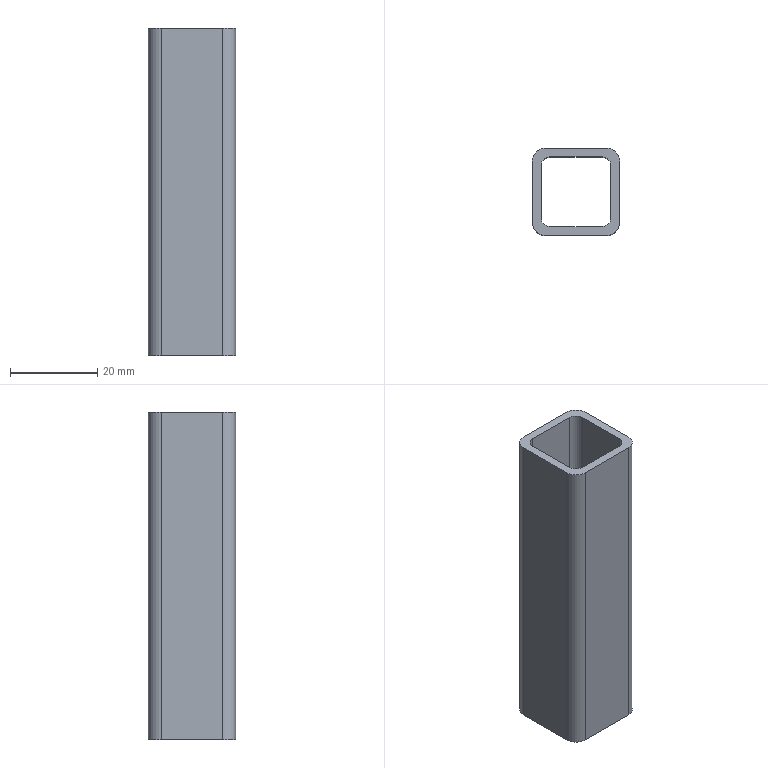Part | STEP file | DIN EN 10210-2 - 20 x 20 x 2 - 100 | 1 solid | 18 faces | box 20 x 20 x 75 mm | volume 10478 mm3 | plane 10 | cylinder 8 | commonest cylinder face diameters 4 x4 6 x4
STEP:
#1=CARTESIAN_POINT('',(0.,0.,0.));
#2=DIRECTION('',(0.,0.,1.));
#3=DIRECTION('',(1.,0.,0.));
#4=AXIS2_PLACEMENT_3D('',#1,#2,#3);
#5=CARTESIAN_POINT('',(8.,6.,0.));
#6=VERTEX_POINT('',#5);
#7=CARTESIAN_POINT('',(8.,6.,75.));
#8=VERTEX_POINT('',#7);
#9=CARTESIAN_POINT('',(8.,6.,0.));
#10=DIRECTION('',(0.,0.,1.));
#11=VECTOR('',#10,1.);
#12=LINE('',#9,#11);
#13=CARTESIAN_POINT('',(6.,6.,0.));
#14=DIRECTION('',(0.,0.,1.));
#15=DIRECTION('',(1.,0.,0.));
#16=AXIS2_PLACEMENT_3D('',#13,#14,#15);
#17=CYLINDRICAL_SURFACE('',#16,2.);
#18=CARTESIAN_POINT('',(0.,0.));
#19=DIRECTION('',(0.,1.));
#20=VECTOR('',#19,1.);
#21=LINE('',#18,#20);
#22=(GEOMETRIC_REPRESENTATION_CONTEXT(2)PARAMETRIC_REPRESENTATION_CONTEXT()REPRESENTATION_CONTEXT('',''));
#23=DEFINITIONAL_REPRESENTATION('',(#21),#22);
#24=PCURVE('',#17,#23);
#25=CARTESIAN_POINT('',(8.,6.,0.));
#26=DIRECTION('',(1.,0.,0.));
#27=DIRECTION('',(0.,0.,-1.));
#28=AXIS2_PLACEMENT_3D('',#25,#26,#27);
#29=PLANE('',#28);
#30=CARTESIAN_POINT('',(0.,0.));
#31=DIRECTION('',(-1.,0.));
#32=VECTOR('',#31,1.);
#33=LINE('',#30,#32);
#34=(GEOMETRIC_REPRESENTATION_CONTEXT(2)PARAMETRIC_REPRESENTATION_CONTEXT()REPRESENTATION_CONTEXT('',''));
#35=DEFINITIONAL_REPRESENTATION('',(#33),#34);
#36=PCURVE('',#29,#35);
#37=SURFACE_CURVE('',#12,(#24,#36),.PCURVE_S1.);
#38=EDGE_CURVE('',#6,#8,#37,.T.);
#39=ORIENTED_EDGE('',*,*,#38,.F.);
#40=CARTESIAN_POINT('',(6.,8.,0.));
#41=VERTEX_POINT('',#40);
#42=CARTESIAN_POINT('',(6.,6.,0.));
#43=DIRECTION('',(0.,0.,1.));
#44=DIRECTION('',(1.,0.,0.));
#45=AXIS2_PLACEMENT_3D('',#42,#43,#44);
#46=CIRCLE('',#45,2.);
#47=CARTESIAN_POINT('',(0.,0.));
#48=DIRECTION('',(1.,0.));
#49=VECTOR('',#48,1.);
#50=LINE('',#47,#49);
#51=(GEOMETRIC_REPRESENTATION_CONTEXT(2)PARAMETRIC_REPRESENTATION_CONTEXT()REPRESENTATION_CONTEXT('',''));
#52=DEFINITIONAL_REPRESENTATION('',(#50),#51);
#53=PCURVE('',#17,#52);
#54=CARTESIAN_POINT('',(0.,0.,0.));
#55=DIRECTION('',(0.,0.,1.));
#56=DIRECTION('',(1.,0.,0.));
#57=AXIS2_PLACEMENT_3D('',#54,#55,#56);
#58=PLANE('',#57);
#59=CARTESIAN_POINT('',(6.,6.));
#60=DIRECTION('',(1.,0.));
#61=AXIS2_PLACEMENT_2D('',#59,#60);
#62=CIRCLE('',#61,2.);
#63=(GEOMETRIC_REPRESENTATION_CONTEXT(2)PARAMETRIC_REPRESENTATION_CONTEXT()REPRESENTATION_CONTEXT('',''));
#64=DEFINITIONAL_REPRESENTATION('',(#62),#63);
#65=PCURVE('',#58,#64);
#66=SURFACE_CURVE('',#46,(#53,#65),.PCURVE_S1.);
#67=EDGE_CURVE('',#6,#41,#66,.T.);
#68=ORIENTED_EDGE('',*,*,#67,.T.);
#69=CARTESIAN_POINT('',(6.,8.,75.));
#70=VERTEX_POINT('',#69);
#71=CARTESIAN_POINT('',(6.,8.,0.));
#72=DIRECTION('',(0.,0.,1.));
#73=VECTOR('',#72,1.);
#74=LINE('',#71,#73);
#75=CARTESIAN_POINT('',(1.571,0.));
#76=DIRECTION('',(0.,1.));
#77=VECTOR('',#76,1.);
#78=LINE('',#75,#77);
#79=(GEOMETRIC_REPRESENTATION_CONTEXT(2)PARAMETRIC_REPRESENTATION_CONTEXT()REPRESENTATION_CONTEXT('',''));
#80=DEFINITIONAL_REPRESENTATION('',(#78),#79);
#81=PCURVE('',#17,#80);
#82=CARTESIAN_POINT('',(-6.,8.,0.));
#83=DIRECTION('',(0.,1.,0.));
#84=DIRECTION('',(0.,0.,1.));
#85=AXIS2_PLACEMENT_3D('',#82,#83,#84);
#86=PLANE('',#85);
#87=CARTESIAN_POINT('',(0.,12.));
#88=DIRECTION('',(1.,0.));
#89=VECTOR('',#88,1.);
#90=LINE('',#87,#89);
#91=(GEOMETRIC_REPRESENTATION_CONTEXT(2)PARAMETRIC_REPRESENTATION_CONTEXT()REPRESENTATION_CONTEXT('',''));
#92=DEFINITIONAL_REPRESENTATION('',(#90),#91);
#93=PCURVE('',#86,#92);
#94=SURFACE_CURVE('',#74,(#81,#93),.PCURVE_S1.);
#95=EDGE_CURVE('',#41,#70,#94,.T.);
#96=ORIENTED_EDGE('',*,*,#95,.T.);
#97=CARTESIAN_POINT('',(6.,6.,75.));
#98=DIRECTION('',(0.,0.,1.));
#99=DIRECTION('',(1.,0.,0.));
#100=AXIS2_PLACEMENT_3D('',#97,#98,#99);
#101=CIRCLE('',#100,2.);
#102=CARTESIAN_POINT('',(0.,75.));
#103=DIRECTION('',(1.,0.));
#104=VECTOR('',#103,1.);
#105=LINE('',#102,#104);
#106=(GEOMETRIC_REPRESENTATION_CONTEXT(2)PARAMETRIC_REPRESENTATION_CONTEXT()REPRESENTATION_CONTEXT('',''));
#107=DEFINITIONAL_REPRESENTATION('',(#105),#106);
#108=PCURVE('',#17,#107);
#109=CARTESIAN_POINT('',(0.,0.,75.));
#110=DIRECTION('',(0.,0.,1.));
#111=DIRECTION('',(1.,0.,0.));
#112=AXIS2_PLACEMENT_3D('',#109,#110,#111);
#113=PLANE('',#112);
#114=CARTESIAN_POINT('',(6.,6.));
#115=DIRECTION('',(1.,0.));
#116=AXIS2_PLACEMENT_2D('',#114,#115);
#117=CIRCLE('',#116,2.);
#118=(GEOMETRIC_REPRESENTATION_CONTEXT(2)PARAMETRIC_REPRESENTATION_CONTEXT()REPRESENTATION_CONTEXT('',''));
#119=DEFINITIONAL_REPRESENTATION('',(#117),#118);
#120=PCURVE('',#113,#119);
#121=SURFACE_CURVE('',#101,(#108,#120),.PCURVE_S1.);
#122=EDGE_CURVE('',#8,#70,#121,.T.);
#123=ORIENTED_EDGE('',*,*,#122,.F.);
#124=EDGE_LOOP('',(#39,#68,#96,#123));
#125=FACE_BOUND('',#124,.F.);
#126=ADVANCED_FACE('',(#125),#17,.F.);
#127=CARTESIAN_POINT('',(-6.,8.,75.));
#128=VERTEX_POINT('',#127);
#129=CARTESIAN_POINT('',(-3.,8.,75.));
#130=DIRECTION('',(-1.,0.,0.));
#131=VECTOR('',#130,1.);
#132=LINE('',#129,#131);
#133=CARTESIAN_POINT('',(75.,3.));
#134=DIRECTION('',(0.,-1.));
#135=VECTOR('',#134,1.);
#136=LINE('',#133,#135);
#137=(GEOMETRIC_REPRESENTATION_CONTEXT(2)PARAMETRIC_REPRESENTATION_CONTEXT()REPRESENTATION_CONTEXT('',''));
#138=DEFINITIONAL_REPRESENTATION('',(#136),#137);
#139=PCURVE('',#86,#138);
#140=CARTESIAN_POINT('',(-3.,8.));
#141=DIRECTION('',(-1.,0.));
#142=VECTOR('',#141,1.);
#143=LINE('',#140,#142);
#144=(GEOMETRIC_REPRESENTATION_CONTEXT(2)PARAMETRIC_REPRESENTATION_CONTEXT()REPRESENTATION_CONTEXT('',''));
#145=DEFINITIONAL_REPRESENTATION('',(#143),#144);
#146=PCURVE('',#113,#145);
#147=SURFACE_CURVE('',#132,(#139,#146),.PCURVE_S1.);
#148=EDGE_CURVE('',#70,#128,#147,.T.);
#149=ORIENTED_EDGE('',*,*,#148,.T.);
#150=CARTESIAN_POINT('',(-6.,8.,0.));
#151=VERTEX_POINT('',#150);
#152=CARTESIAN_POINT('',(-6.,8.,0.));
#153=DIRECTION('',(0.,0.,1.));
#154=VECTOR('',#153,1.);
#155=LINE('',#152,#154);
#156=CARTESIAN_POINT('',(0.,0.));
#157=DIRECTION('',(1.,0.));
#158=VECTOR('',#157,1.);
#159=LINE('',#156,#158);
#160=(GEOMETRIC_REPRESENTATION_CONTEXT(2)PARAMETRIC_REPRESENTATION_CONTEXT()REPRESENTATION_CONTEXT('',''));
#161=DEFINITIONAL_REPRESENTATION('',(#159),#160);
#162=PCURVE('',#86,#161);
#163=CARTESIAN_POINT('',(-6.,6.,0.));
#164=DIRECTION('',(0.,0.,1.));
#165=DIRECTION('',(0.,1.,0.));
#166=AXIS2_PLACEMENT_3D('',#163,#164,#165);
#167=CYLINDRICAL_SURFACE('',#166,2.);
#168=CARTESIAN_POINT('',(0.,0.));
#169=DIRECTION('',(0.,1.));
#170=VECTOR('',#169,1.);
#171=LINE('',#168,#170);
#172=(GEOMETRIC_REPRESENTATION_CONTEXT(2)PARAMETRIC_REPRESENTATION_CONTEXT()REPRESENTATION_CONTEXT('',''));
#173=DEFINITIONAL_REPRESENTATION('',(#171),#172);
#174=PCURVE('',#167,#173);
#175=SURFACE_CURVE('',#155,(#162,#174),.PCURVE_S1.);
#176=EDGE_CURVE('',#151,#128,#175,.T.);
#177=ORIENTED_EDGE('',*,*,#176,.F.);
#178=CARTESIAN_POINT('',(-3.,8.,0.));
#179=DIRECTION('',(-1.,0.,0.));
#180=VECTOR('',#179,1.);
#181=LINE('',#178,#180);
#182=CARTESIAN_POINT('',(0.,3.));
#183=DIRECTION('',(0.,-1.));
#184=VECTOR('',#183,1.);
#185=LINE('',#182,#184);
#186=(GEOMETRIC_REPRESENTATION_CONTEXT(2)PARAMETRIC_REPRESENTATION_CONTEXT()REPRESENTATION_CONTEXT('',''));
#187=DEFINITIONAL_REPRESENTATION('',(#185),#186);
#188=PCURVE('',#86,#187);
#189=CARTESIAN_POINT('',(-3.,8.));
#190=DIRECTION('',(-1.,0.));
#191=VECTOR('',#190,1.);
#192=LINE('',#189,#191);
#193=(GEOMETRIC_REPRESENTATION_CONTEXT(2)PARAMETRIC_REPRESENTATION_CONTEXT()REPRESENTATION_CONTEXT('',''));
#194=DEFINITIONAL_REPRESENTATION('',(#192),#193);
#195=PCURVE('',#58,#194);
#196=SURFACE_CURVE('',#181,(#188,#195),.PCURVE_S1.);
#197=EDGE_CURVE('',#41,#151,#196,.T.);
#198=ORIENTED_EDGE('',*,*,#197,.F.);
#199=ORIENTED_EDGE('',*,*,#95,.T.);
#200=EDGE_LOOP('',(#149,#177,#198,#199));
#201=FACE_BOUND('',#200,.T.);
#202=ADVANCED_FACE('',(#201),#86,.F.);
#203=ORIENTED_EDGE('',*,*,#176,.F.);
#204=CARTESIAN_POINT('',(-8.,6.,0.));
#205=VERTEX_POINT('',#204);
#206=CARTESIAN_POINT('',(-6.,6.,0.));
#207=DIRECTION('',(0.,0.,1.));
#208=DIRECTION('',(0.,1.,0.));
#209=AXIS2_PLACEMENT_3D('',#206,#207,#208);
#210=CIRCLE('',#209,2.);
#211=CARTESIAN_POINT('',(0.,0.));
#212=DIRECTION('',(1.,0.));
#213=VECTOR('',#212,1.);
#214=LINE('',#211,#213);
#215=(GEOMETRIC_REPRESENTATION_CONTEXT(2)PARAMETRIC_REPRESENTATION_CONTEXT()REPRESENTATION_CONTEXT('',''));
#216=DEFINITIONAL_REPRESENTATION('',(#214),#215);
#217=PCURVE('',#167,#216);
#218=CARTESIAN_POINT('',(-6.,6.));
#219=DIRECTION('',(0.,1.));
#220=AXIS2_PLACEMENT_2D('',#218,#219);
#221=CIRCLE('',#220,2.);
#222=(GEOMETRIC_REPRESENTATION_CONTEXT(2)PARAMETRIC_REPRESENTATION_CONTEXT()REPRESENTATION_CONTEXT('',''));
#223=DEFINITIONAL_REPRESENTATION('',(#221),#222);
#224=PCURVE('',#58,#223);
#225=SURFACE_CURVE('',#210,(#217,#224),.PCURVE_S1.);
#226=EDGE_CURVE('',#151,#205,#225,.T.);
#227=ORIENTED_EDGE('',*,*,#226,.T.);
#228=CARTESIAN_POINT('',(-8.,6.,75.));
#229=VERTEX_POINT('',#228);
#230=CARTESIAN_POINT('',(-8.,6.,0.));
#231=DIRECTION('',(0.,0.,1.));
#232=VECTOR('',#231,1.);
#233=LINE('',#230,#232);
#234=CARTESIAN_POINT('',(1.571,0.));
#235=DIRECTION('',(0.,1.));
#236=VECTOR('',#235,1.);
#237=LINE('',#234,#236);
#238=(GEOMETRIC_REPRESENTATION_CONTEXT(2)PARAMETRIC_REPRESENTATION_CONTEXT()REPRESENTATION_CONTEXT('',''));
#239=DEFINITIONAL_REPRESENTATION('',(#237),#238);
#240=PCURVE('',#167,#239);
#241=CARTESIAN_POINT('',(-8.,-6.,0.));
#242=DIRECTION('',(-1.,0.,0.));
#243=DIRECTION('',(0.,0.,1.));
#244=AXIS2_PLACEMENT_3D('',#241,#242,#243);
#245=PLANE('',#244);
#246=CARTESIAN_POINT('',(0.,12.));
#247=DIRECTION('',(1.,0.));
#248=VECTOR('',#247,1.);
#249=LINE('',#246,#248);
#250=(GEOMETRIC_REPRESENTATION_CONTEXT(2)PARAMETRIC_REPRESENTATION_CONTEXT()REPRESENTATION_CONTEXT('',''));
#251=DEFINITIONAL_REPRESENTATION('',(#249),#250);
#252=PCURVE('',#245,#251);
#253=SURFACE_CURVE('',#233,(#240,#252),.PCURVE_S1.);
#254=EDGE_CURVE('',#205,#229,#253,.T.);
#255=ORIENTED_EDGE('',*,*,#254,.T.);
#256=CARTESIAN_POINT('',(-6.,6.,75.));
#257=DIRECTION('',(0.,0.,1.));
#258=DIRECTION('',(0.,1.,0.));
#259=AXIS2_PLACEMENT_3D('',#256,#257,#258);
#260=CIRCLE('',#259,2.);
#261=CARTESIAN_POINT('',(0.,75.));
#262=DIRECTION('',(1.,0.));
#263=VECTOR('',#262,1.);
#264=LINE('',#261,#263);
#265=(GEOMETRIC_REPRESENTATION_CONTEXT(2)PARAMETRIC_REPRESENTATION_CONTEXT()REPRESENTATION_CONTEXT('',''));
#266=DEFINITIONAL_REPRESENTATION('',(#264),#265);
#267=PCURVE('',#167,#266);
#268=CARTESIAN_POINT('',(-6.,6.));
#269=DIRECTION('',(0.,1.));
#270=AXIS2_PLACEMENT_2D('',#268,#269);
#271=CIRCLE('',#270,2.);
#272=(GEOMETRIC_REPRESENTATION_CONTEXT(2)PARAMETRIC_REPRESENTATION_CONTEXT()REPRESENTATION_CONTEXT('',''));
#273=DEFINITIONAL_REPRESENTATION('',(#271),#272);
#274=PCURVE('',#113,#273);
#275=SURFACE_CURVE('',#260,(#267,#274),.PCURVE_S1.);
#276=EDGE_CURVE('',#128,#229,#275,.T.);
#277=ORIENTED_EDGE('',*,*,#276,.F.);
#278=EDGE_LOOP('',(#203,#227,#255,#277));
#279=FACE_BOUND('',#278,.F.);
#280=ADVANCED_FACE('',(#279),#167,.F.);
#281=CARTESIAN_POINT('',(-8.,-6.,75.));
#282=VERTEX_POINT('',#281);
#283=CARTESIAN_POINT('',(-8.,-3.,75.));
#284=DIRECTION('',(0.,-1.,0.));
#285=VECTOR('',#284,1.);
#286=LINE('',#283,#285);
#287=CARTESIAN_POINT('',(75.,3.));
#288=DIRECTION('',(0.,-1.));
#289=VECTOR('',#288,1.);
#290=LINE('',#287,#289);
#291=(GEOMETRIC_REPRESENTATION_CONTEXT(2)PARAMETRIC_REPRESENTATION_CONTEXT()REPRESENTATION_CONTEXT('',''));
#292=DEFINITIONAL_REPRESENTATION('',(#290),#291);
#293=PCURVE('',#245,#292);
#294=CARTESIAN_POINT('',(-8.,-3.));
#295=DIRECTION('',(0.,-1.));
#296=VECTOR('',#295,1.);
#297=LINE('',#294,#296);
#298=(GEOMETRIC_REPRESENTATION_CONTEXT(2)PARAMETRIC_REPRESENTATION_CONTEXT()REPRESENTATION_CONTEXT('',''));
#299=DEFINITIONAL_REPRESENTATION('',(#297),#298);
#300=PCURVE('',#113,#299);
#301=SURFACE_CURVE('',#286,(#293,#300),.PCURVE_S1.);
#302=EDGE_CURVE('',#229,#282,#301,.T.);
#303=ORIENTED_EDGE('',*,*,#302,.T.);
#304=CARTESIAN_POINT('',(-8.,-6.,0.));
#305=VERTEX_POINT('',#304);
#306=CARTESIAN_POINT('',(-8.,-6.,0.));
#307=DIRECTION('',(0.,0.,1.));
#308=VECTOR('',#307,1.);
#309=LINE('',#306,#308);
#310=CARTESIAN_POINT('',(0.,0.));
#311=DIRECTION('',(1.,0.));
#312=VECTOR('',#311,1.);
#313=LINE('',#310,#312);
#314=(GEOMETRIC_REPRESENTATION_CONTEXT(2)PARAMETRIC_REPRESENTATION_CONTEXT()REPRESENTATION_CONTEXT('',''));
#315=DEFINITIONAL_REPRESENTATION('',(#313),#314);
#316=PCURVE('',#245,#315);
#317=CARTESIAN_POINT('',(-6.,-6.,0.));
#318=DIRECTION('',(0.,0.,1.));
#319=DIRECTION('',(-1.,0.,0.));
#320=AXIS2_PLACEMENT_3D('',#317,#318,#319);
#321=CYLINDRICAL_SURFACE('',#320,2.);
#322=CARTESIAN_POINT('',(0.,0.));
#323=DIRECTION('',(0.,1.));
#324=VECTOR('',#323,1.);
#325=LINE('',#322,#324);
#326=(GEOMETRIC_REPRESENTATION_CONTEXT(2)PARAMETRIC_REPRESENTATION_CONTEXT()REPRESENTATION_CONTEXT('',''));
#327=DEFINITIONAL_REPRESENTATION('',(#325),#326);
#328=PCURVE('',#321,#327);
#329=SURFACE_CURVE('',#309,(#316,#328),.PCURVE_S1.);
#330=EDGE_CURVE('',#305,#282,#329,.T.);
#331=ORIENTED_EDGE('',*,*,#330,.F.);
#332=CARTESIAN_POINT('',(-8.,-3.,0.));
#333=DIRECTION('',(0.,-1.,0.));
#334=VECTOR('',#333,1.);
#335=LINE('',#332,#334);
#336=CARTESIAN_POINT('',(0.,3.));
#337=DIRECTION('',(0.,-1.));
#338=VECTOR('',#337,1.);
#339=LINE('',#336,#338);
#340=(GEOMETRIC_REPRESENTATION_CONTEXT(2)PARAMETRIC_REPRESENTATION_CONTEXT()REPRESENTATION_CONTEXT('',''));
#341=DEFINITIONAL_REPRESENTATION('',(#339),#340);
#342=PCURVE('',#245,#341);
#343=CARTESIAN_POINT('',(-8.,-3.));
#344=DIRECTION('',(0.,-1.));
#345=VECTOR('',#344,1.);
#346=LINE('',#343,#345);
#347=(GEOMETRIC_REPRESENTATION_CONTEXT(2)PARAMETRIC_REPRESENTATION_CONTEXT()REPRESENTATION_CONTEXT('',''));
#348=DEFINITIONAL_REPRESENTATION('',(#346),#347);
#349=PCURVE('',#58,#348);
#350=SURFACE_CURVE('',#335,(#342,#349),.PCURVE_S1.);
#351=EDGE_CURVE('',#205,#305,#350,.T.);
#352=ORIENTED_EDGE('',*,*,#351,.F.);
#353=ORIENTED_EDGE('',*,*,#254,.T.);
#354=EDGE_LOOP('',(#303,#331,#352,#353));
#355=FACE_BOUND('',#354,.T.);
#356=ADVANCED_FACE('',(#355),#245,.F.);
#357=CARTESIAN_POINT('',(10.,7.,75.));
#358=VERTEX_POINT('',#357);
#359=CARTESIAN_POINT('',(10.,-7.,75.));
#360=VERTEX_POINT('',#359);
#361=CARTESIAN_POINT('',(10.,3.5,75.));
#362=DIRECTION('',(0.,-1.,0.));
#363=VECTOR('',#362,1.);
#364=LINE('',#361,#363);
#365=CARTESIAN_POINT('',(10.,7.,0.));
#366=DIRECTION('',(1.,0.,0.));
#367=DIRECTION('',(0.,0.,-1.));
#368=AXIS2_PLACEMENT_3D('',#365,#366,#367);
#369=PLANE('',#368);
#370=CARTESIAN_POINT('',(-75.,-3.5));
#371=DIRECTION('',(0.,-1.));
#372=VECTOR('',#371,1.);
#373=LINE('',#370,#372);
#374=(GEOMETRIC_REPRESENTATION_CONTEXT(2)PARAMETRIC_REPRESENTATION_CONTEXT()REPRESENTATION_CONTEXT('',''));
#375=DEFINITIONAL_REPRESENTATION('',(#373),#374);
#376=PCURVE('',#369,#375);
#377=CARTESIAN_POINT('',(10.,3.5));
#378=DIRECTION('',(0.,-1.));
#379=VECTOR('',#378,1.);
#380=LINE('',#377,#379);
#381=(GEOMETRIC_REPRESENTATION_CONTEXT(2)PARAMETRIC_REPRESENTATION_CONTEXT()REPRESENTATION_CONTEXT('',''));
#382=DEFINITIONAL_REPRESENTATION('',(#380),#381);
#383=PCURVE('',#113,#382);
#384=SURFACE_CURVE('',#364,(#376,#383),.PCURVE_S1.);
#385=EDGE_CURVE('',#358,#360,#384,.T.);
#386=ORIENTED_EDGE('',*,*,#385,.T.);
#387=CARTESIAN_POINT('',(10.,-7.,0.));
#388=VERTEX_POINT('',#387);
#389=CARTESIAN_POINT('',(10.,-7.,0.));
#390=DIRECTION('',(0.,0.,1.));
#391=VECTOR('',#390,1.);
#392=LINE('',#389,#391);
#393=CARTESIAN_POINT('',(0.,-14.));
#394=DIRECTION('',(-1.,0.));
#395=VECTOR('',#394,1.);
#396=LINE('',#393,#395);
#397=(GEOMETRIC_REPRESENTATION_CONTEXT(2)PARAMETRIC_REPRESENTATION_CONTEXT()REPRESENTATION_CONTEXT('',''));
#398=DEFINITIONAL_REPRESENTATION('',(#396),#397);
#399=PCURVE('',#369,#398);
#400=CARTESIAN_POINT('',(7.,-7.,0.));
#401=DIRECTION('',(0.,0.,1.));
#402=DIRECTION('',(0.,1.,0.));
#403=AXIS2_PLACEMENT_3D('',#400,#401,#402);
#404=CYLINDRICAL_SURFACE('',#403,3.);
#405=CARTESIAN_POINT('',(4.712,0.));
#406=DIRECTION('',(0.,1.));
#407=VECTOR('',#406,1.);
#408=LINE('',#405,#407);
#409=(GEOMETRIC_REPRESENTATION_CONTEXT(2)PARAMETRIC_REPRESENTATION_CONTEXT()REPRESENTATION_CONTEXT('',''));
#410=DEFINITIONAL_REPRESENTATION('',(#408),#409);
#411=PCURVE('',#404,#410);
#412=SURFACE_CURVE('',#392,(#399,#411),.PCURVE_S1.);
#413=EDGE_CURVE('',#388,#360,#412,.T.);
#414=ORIENTED_EDGE('',*,*,#413,.F.);
#415=CARTESIAN_POINT('',(10.,7.,0.));
#416=VERTEX_POINT('',#415);
#417=CARTESIAN_POINT('',(10.,3.5,0.));
#418=DIRECTION('',(0.,-1.,0.));
#419=VECTOR('',#418,1.);
#420=LINE('',#417,#419);
#421=CARTESIAN_POINT('',(0.,-3.5));
#422=DIRECTION('',(0.,-1.));
#423=VECTOR('',#422,1.);
#424=LINE('',#421,#423);
#425=(GEOMETRIC_REPRESENTATION_CONTEXT(2)PARAMETRIC_REPRESENTATION_CONTEXT()REPRESENTATION_CONTEXT('',''));
#426=DEFINITIONAL_REPRESENTATION('',(#424),#425);
#427=PCURVE('',#369,#426);
#428=CARTESIAN_POINT('',(10.,3.5));
#429=DIRECTION('',(0.,-1.));
#430=VECTOR('',#429,1.);
#431=LINE('',#428,#430);
#432=(GEOMETRIC_REPRESENTATION_CONTEXT(2)PARAMETRIC_REPRESENTATION_CONTEXT()REPRESENTATION_CONTEXT('',''));
#433=DEFINITIONAL_REPRESENTATION('',(#431),#432);
#434=PCURVE('',#58,#433);
#435=SURFACE_CURVE('',#420,(#427,#434),.PCURVE_S1.);
#436=EDGE_CURVE('',#416,#388,#435,.T.);
#437=ORIENTED_EDGE('',*,*,#436,.F.);
#438=CARTESIAN_POINT('',(10.,7.,0.));
#439=DIRECTION('',(0.,0.,1.));
#440=VECTOR('',#439,1.);
#441=LINE('',#438,#440);
#442=CARTESIAN_POINT('',(0.,0.));
#443=DIRECTION('',(-1.,0.));
#444=VECTOR('',#443,1.);
#445=LINE('',#442,#444);
#446=(GEOMETRIC_REPRESENTATION_CONTEXT(2)PARAMETRIC_REPRESENTATION_CONTEXT()REPRESENTATION_CONTEXT('',''));
#447=DEFINITIONAL_REPRESENTATION('',(#445),#446);
#448=PCURVE('',#369,#447);
#449=CARTESIAN_POINT('',(7.,7.,0.));
#450=DIRECTION('',(0.,0.,1.));
#451=DIRECTION('',(-1.,0.,0.));
#452=AXIS2_PLACEMENT_3D('',#449,#450,#451);
#453=CYLINDRICAL_SURFACE('',#452,3.);
#454=CARTESIAN_POINT('',(3.142,0.));
#455=DIRECTION('',(0.,1.));
#456=VECTOR('',#455,1.);
#457=LINE('',#454,#456);
#458=(GEOMETRIC_REPRESENTATION_CONTEXT(2)PARAMETRIC_REPRESENTATION_CONTEXT()REPRESENTATION_CONTEXT('',''));
#459=DEFINITIONAL_REPRESENTATION('',(#457),#458);
#460=PCURVE('',#453,#459);
#461=SURFACE_CURVE('',#441,(#448,#460),.PCURVE_S1.);
#462=EDGE_CURVE('',#416,#358,#461,.T.);
#463=ORIENTED_EDGE('',*,*,#462,.T.);
#464=EDGE_LOOP('',(#386,#414,#437,#463));
#465=FACE_BOUND('',#464,.T.);
#466=ADVANCED_FACE('',(#465),#369,.T.);
#467=CARTESIAN_POINT('',(7.,-10.,75.));
#468=VERTEX_POINT('',#467);
#469=CARTESIAN_POINT('',(7.,-7.,75.));
#470=DIRECTION('',(0.,0.,-1.));
#471=DIRECTION('',(0.,1.,0.));
#472=AXIS2_PLACEMENT_3D('',#469,#470,#471);
#473=CIRCLE('',#472,3.);
#474=CARTESIAN_POINT('',(6.283,75.));
#475=DIRECTION('',(-1.,0.));
#476=VECTOR('',#475,1.);
#477=LINE('',#474,#476);
#478=(GEOMETRIC_REPRESENTATION_CONTEXT(2)PARAMETRIC_REPRESENTATION_CONTEXT()REPRESENTATION_CONTEXT('',''));
#479=DEFINITIONAL_REPRESENTATION('',(#477),#478);
#480=PCURVE('',#404,#479);
#481=CARTESIAN_POINT('',(7.,-4.));
#482=CARTESIAN_POINT('',(12.196,-4.));
#483=CARTESIAN_POINT('',(9.598,-8.5));
#484=CARTESIAN_POINT('',(7.,-13.));
#485=CARTESIAN_POINT('',(4.402,-8.5));
#486=CARTESIAN_POINT('',(1.804,-4.));
#487=CARTESIAN_POINT('',(7.,-4.));
#488=(BOUNDED_CURVE()B_SPLINE_CURVE(2,(#481,#482,#483,#484,#485,#486,#487),.UNSPECIFIED.,.T.,.F.)B_SPLINE_CURVE_WITH_KNOTS((1,2,2,2,2,1),(-2.094,0.,2.094,4.189,6.283,8.378),.UNSPECIFIED.)CURVE()GEOMETRIC_REPRESENTATION_ITEM()RATIONAL_B_SPLINE_CURVE((1.,0.5,1.,0.5,1.,0.5,1.))REPRESENTATION_ITEM(''));
#489=(GEOMETRIC_REPRESENTATION_CONTEXT(2)PARAMETRIC_REPRESENTATION_CONTEXT()REPRESENTATION_CONTEXT('',''));
#490=DEFINITIONAL_REPRESENTATION('',(#488),#489);
#491=PCURVE('',#113,#490);
#492=SURFACE_CURVE('',#473,(#480,#491),.PCURVE_S1.);
#493=EDGE_CURVE('',#360,#468,#492,.T.);
#494=ORIENTED_EDGE('',*,*,#493,.T.);
#495=CARTESIAN_POINT('',(7.,-10.,0.));
#496=VERTEX_POINT('',#495);
#497=CARTESIAN_POINT('',(7.,-10.,0.));
#498=DIRECTION('',(0.,0.,1.));
#499=VECTOR('',#498,1.);
#500=LINE('',#497,#499);
#501=CARTESIAN_POINT('',(3.142,0.));
#502=DIRECTION('',(0.,1.));
#503=VECTOR('',#502,1.);
#504=LINE('',#501,#503);
#505=(GEOMETRIC_REPRESENTATION_CONTEXT(2)PARAMETRIC_REPRESENTATION_CONTEXT()REPRESENTATION_CONTEXT('',''));
#506=DEFINITIONAL_REPRESENTATION('',(#504),#505);
#507=PCURVE('',#404,#506);
#508=CARTESIAN_POINT('',(7.,-10.,0.));
#509=DIRECTION('',(0.,-1.,0.));
#510=DIRECTION('',(0.,0.,-1.));
#511=AXIS2_PLACEMENT_3D('',#508,#509,#510);
#512=PLANE('',#511);
#513=CARTESIAN_POINT('',(0.,0.));
#514=DIRECTION('',(-1.,0.));
#515=VECTOR('',#514,1.);
#516=LINE('',#513,#515);
#517=(GEOMETRIC_REPRESENTATION_CONTEXT(2)PARAMETRIC_REPRESENTATION_CONTEXT()REPRESENTATION_CONTEXT('',''));
#518=DEFINITIONAL_REPRESENTATION('',(#516),#517);
#519=PCURVE('',#512,#518);
#520=SURFACE_CURVE('',#500,(#507,#519),.PCURVE_S1.);
#521=EDGE_CURVE('',#496,#468,#520,.T.);
#522=ORIENTED_EDGE('',*,*,#521,.F.);
#523=CARTESIAN_POINT('',(7.,-7.,0.));
#524=DIRECTION('',(0.,0.,-1.));
#525=DIRECTION('',(0.,1.,0.));
#526=AXIS2_PLACEMENT_3D('',#523,#524,#525);
#527=CIRCLE('',#526,3.);
#528=CARTESIAN_POINT('',(6.283,0.));
#529=DIRECTION('',(-1.,0.));
#530=VECTOR('',#529,1.);
#531=LINE('',#528,#530);
#532=(GEOMETRIC_REPRESENTATION_CONTEXT(2)PARAMETRIC_REPRESENTATION_CONTEXT()REPRESENTATION_CONTEXT('',''));
#533=DEFINITIONAL_REPRESENTATION('',(#531),#532);
#534=PCURVE('',#404,#533);
#535=CARTESIAN_POINT('',(7.,-4.));
#536=CARTESIAN_POINT('',(12.196,-4.));
#537=CARTESIAN_POINT('',(9.598,-8.5));
#538=CARTESIAN_POINT('',(7.,-13.));
#539=CARTESIAN_POINT('',(4.402,-8.5));
#540=CARTESIAN_POINT('',(1.804,-4.));
#541=CARTESIAN_POINT('',(7.,-4.));
#542=(BOUNDED_CURVE()B_SPLINE_CURVE(2,(#535,#536,#537,#538,#539,#540,#541),.UNSPECIFIED.,.T.,.F.)B_SPLINE_CURVE_WITH_KNOTS((1,2,2,2,2,1),(-2.094,0.,2.094,4.189,6.283,8.378),.UNSPECIFIED.)CURVE()GEOMETRIC_REPRESENTATION_ITEM()RATIONAL_B_SPLINE_CURVE((1.,0.5,1.,0.5,1.,0.5,1.))REPRESENTATION_ITEM(''));
#543=(GEOMETRIC_REPRESENTATION_CONTEXT(2)PARAMETRIC_REPRESENTATION_CONTEXT()REPRESENTATION_CONTEXT('',''));
#544=DEFINITIONAL_REPRESENTATION('',(#542),#543);
#545=PCURVE('',#58,#544);
#546=SURFACE_CURVE('',#527,(#534,#545),.PCURVE_S1.);
#547=EDGE_CURVE('',#388,#496,#546,.T.);
#548=ORIENTED_EDGE('',*,*,#547,.F.);
#549=ORIENTED_EDGE('',*,*,#413,.T.);
#550=EDGE_LOOP('',(#494,#522,#548,#549));
#551=FACE_BOUND('',#550,.T.);
#552=ADVANCED_FACE('',(#551),#404,.T.);
#553=CARTESIAN_POINT('',(-7.,-10.,75.));
#554=VERTEX_POINT('',#553);
#555=CARTESIAN_POINT('',(3.5,-10.,75.));
#556=DIRECTION('',(-1.,0.,0.));
#557=VECTOR('',#556,1.);
#558=LINE('',#555,#557);
#559=CARTESIAN_POINT('',(-75.,-3.5));
#560=DIRECTION('',(0.,-1.));
#561=VECTOR('',#560,1.);
#562=LINE('',#559,#561);
#563=(GEOMETRIC_REPRESENTATION_CONTEXT(2)PARAMETRIC_REPRESENTATION_CONTEXT()REPRESENTATION_CONTEXT('',''));
#564=DEFINITIONAL_REPRESENTATION('',(#562),#563);
#565=PCURVE('',#512,#564);
#566=CARTESIAN_POINT('',(3.5,-10.));
#567=DIRECTION('',(-1.,0.));
#568=VECTOR('',#567,1.);
#569=LINE('',#566,#568);
#570=(GEOMETRIC_REPRESENTATION_CONTEXT(2)PARAMETRIC_REPRESENTATION_CONTEXT()REPRESENTATION_CONTEXT('',''));
#571=DEFINITIONAL_REPRESENTATION('',(#569),#570);
#572=PCURVE('',#113,#571);
#573=SURFACE_CURVE('',#558,(#565,#572),.PCURVE_S1.);
#574=EDGE_CURVE('',#468,#554,#573,.T.);
#575=ORIENTED_EDGE('',*,*,#574,.T.);
#576=CARTESIAN_POINT('',(-7.,-10.,0.));
#577=VERTEX_POINT('',#576);
#578=CARTESIAN_POINT('',(-7.,-10.,0.));
#579=DIRECTION('',(0.,0.,1.));
#580=VECTOR('',#579,1.);
#581=LINE('',#578,#580);
#582=CARTESIAN_POINT('',(0.,-14.));
#583=DIRECTION('',(-1.,0.));
#584=VECTOR('',#583,1.);
#585=LINE('',#582,#584);
#586=(GEOMETRIC_REPRESENTATION_CONTEXT(2)PARAMETRIC_REPRESENTATION_CONTEXT()REPRESENTATION_CONTEXT('',''));
#587=DEFINITIONAL_REPRESENTATION('',(#585),#586);
#588=PCURVE('',#512,#587);
#589=CARTESIAN_POINT('',(-7.,-7.,0.));
#590=DIRECTION('',(0.,0.,1.));
#591=DIRECTION('',(1.,0.,0.));
#592=AXIS2_PLACEMENT_3D('',#589,#590,#591);
#593=CYLINDRICAL_SURFACE('',#592,3.);
#594=CARTESIAN_POINT('',(4.712,0.));
#595=DIRECTION('',(0.,1.));
#596=VECTOR('',#595,1.);
#597=LINE('',#594,#596);
#598=(GEOMETRIC_REPRESENTATION_CONTEXT(2)PARAMETRIC_REPRESENTATION_CONTEXT()REPRESENTATION_CONTEXT('',''));
#599=DEFINITIONAL_REPRESENTATION('',(#597),#598);
#600=PCURVE('',#593,#599);
#601=SURFACE_CURVE('',#581,(#588,#600),.PCURVE_S1.);
#602=EDGE_CURVE('',#577,#554,#601,.T.);
#603=ORIENTED_EDGE('',*,*,#602,.F.);
#604=CARTESIAN_POINT('',(3.5,-10.,0.));
#605=DIRECTION('',(-1.,0.,0.));
#606=VECTOR('',#605,1.);
#607=LINE('',#604,#606);
#608=CARTESIAN_POINT('',(0.,-3.5));
#609=DIRECTION('',(0.,-1.));
#610=VECTOR('',#609,1.);
#611=LINE('',#608,#610);
#612=(GEOMETRIC_REPRESENTATION_CONTEXT(2)PARAMETRIC_REPRESENTATION_CONTEXT()REPRESENTATION_CONTEXT('',''));
#613=DEFINITIONAL_REPRESENTATION('',(#611),#612);
#614=PCURVE('',#512,#613);
#615=CARTESIAN_POINT('',(3.5,-10.));
#616=DIRECTION('',(-1.,0.));
#617=VECTOR('',#616,1.);
#618=LINE('',#615,#617);
#619=(GEOMETRIC_REPRESENTATION_CONTEXT(2)PARAMETRIC_REPRESENTATION_CONTEXT()REPRESENTATION_CONTEXT('',''));
#620=DEFINITIONAL_REPRESENTATION('',(#618),#619);
#621=PCURVE('',#58,#620);
#622=SURFACE_CURVE('',#607,(#614,#621),.PCURVE_S1.);
#623=EDGE_CURVE('',#496,#577,#622,.T.);
#624=ORIENTED_EDGE('',*,*,#623,.F.);
#625=ORIENTED_EDGE('',*,*,#521,.T.);
#626=EDGE_LOOP('',(#575,#603,#624,#625));
#627=FACE_BOUND('',#626,.T.);
#628=ADVANCED_FACE('',(#627),#512,.T.);
#629=CARTESIAN_POINT('',(-10.,-7.,75.));
#630=VERTEX_POINT('',#629);
#631=CARTESIAN_POINT('',(-7.,-7.,75.));
#632=DIRECTION('',(0.,0.,-1.));
#633=DIRECTION('',(1.,0.,0.));
#634=AXIS2_PLACEMENT_3D('',#631,#632,#633);
#635=CIRCLE('',#634,3.);
#636=CARTESIAN_POINT('',(6.283,75.));
#637=DIRECTION('',(-1.,0.));
#638=VECTOR('',#637,1.);
#639=LINE('',#636,#638);
#640=(GEOMETRIC_REPRESENTATION_CONTEXT(2)PARAMETRIC_REPRESENTATION_CONTEXT()REPRESENTATION_CONTEXT('',''));
#641=DEFINITIONAL_REPRESENTATION('',(#639),#640);
#642=PCURVE('',#593,#641);
#643=CARTESIAN_POINT('',(-4.,-7.));
#644=CARTESIAN_POINT('',(-4.,-12.196));
#645=CARTESIAN_POINT('',(-8.5,-9.598));
#646=CARTESIAN_POINT('',(-13.,-7.));
#647=CARTESIAN_POINT('',(-8.5,-4.402));
#648=CARTESIAN_POINT('',(-4.,-1.804));
#649=CARTESIAN_POINT('',(-4.,-7.));
#650=(BOUNDED_CURVE()B_SPLINE_CURVE(2,(#643,#644,#645,#646,#647,#648,#649),.UNSPECIFIED.,.T.,.F.)B_SPLINE_CURVE_WITH_KNOTS((1,2,2,2,2,1),(-2.094,0.,2.094,4.189,6.283,8.378),.UNSPECIFIED.)CURVE()GEOMETRIC_REPRESENTATION_ITEM()RATIONAL_B_SPLINE_CURVE((1.,0.5,1.,0.5,1.,0.5,1.))REPRESENTATION_ITEM(''));
#651=(GEOMETRIC_REPRESENTATION_CONTEXT(2)PARAMETRIC_REPRESENTATION_CONTEXT()REPRESENTATION_CONTEXT('',''));
#652=DEFINITIONAL_REPRESENTATION('',(#650),#651);
#653=PCURVE('',#113,#652);
#654=SURFACE_CURVE('',#635,(#642,#653),.PCURVE_S1.);
#655=EDGE_CURVE('',#554,#630,#654,.T.);
#656=ORIENTED_EDGE('',*,*,#655,.T.);
#657=CARTESIAN_POINT('',(-10.,-7.,0.));
#658=VERTEX_POINT('',#657);
#659=CARTESIAN_POINT('',(-10.,-7.,0.));
#660=DIRECTION('',(0.,0.,1.));
#661=VECTOR('',#660,1.);
#662=LINE('',#659,#661);
#663=CARTESIAN_POINT('',(3.142,0.));
#664=DIRECTION('',(0.,1.));
#665=VECTOR('',#664,1.);
#666=LINE('',#663,#665);
#667=(GEOMETRIC_REPRESENTATION_CONTEXT(2)PARAMETRIC_REPRESENTATION_CONTEXT()REPRESENTATION_CONTEXT('',''));
#668=DEFINITIONAL_REPRESENTATION('',(#666),#667);
#669=PCURVE('',#593,#668);
#670=CARTESIAN_POINT('',(-10.,-7.,0.));
#671=DIRECTION('',(-1.,0.,0.));
#672=DIRECTION('',(0.,0.,1.));
#673=AXIS2_PLACEMENT_3D('',#670,#671,#672);
#674=PLANE('',#673);
#675=CARTESIAN_POINT('',(0.,0.));
#676=DIRECTION('',(1.,0.));
#677=VECTOR('',#676,1.);
#678=LINE('',#675,#677);
#679=(GEOMETRIC_REPRESENTATION_CONTEXT(2)PARAMETRIC_REPRESENTATION_CONTEXT()REPRESENTATION_CONTEXT('',''));
#680=DEFINITIONAL_REPRESENTATION('',(#678),#679);
#681=PCURVE('',#674,#680);
#682=SURFACE_CURVE('',#662,(#669,#681),.PCURVE_S1.);
#683=EDGE_CURVE('',#658,#630,#682,.T.);
#684=ORIENTED_EDGE('',*,*,#683,.F.);
#685=CARTESIAN_POINT('',(-7.,-7.,0.));
#686=DIRECTION('',(0.,0.,-1.));
#687=DIRECTION('',(1.,0.,0.));
#688=AXIS2_PLACEMENT_3D('',#685,#686,#687);
#689=CIRCLE('',#688,3.);
#690=CARTESIAN_POINT('',(6.283,0.));
#691=DIRECTION('',(-1.,0.));
#692=VECTOR('',#691,1.);
#693=LINE('',#690,#692);
#694=(GEOMETRIC_REPRESENTATION_CONTEXT(2)PARAMETRIC_REPRESENTATION_CONTEXT()REPRESENTATION_CONTEXT('',''));
#695=DEFINITIONAL_REPRESENTATION('',(#693),#694);
#696=PCURVE('',#593,#695);
#697=CARTESIAN_POINT('',(-4.,-7.));
#698=CARTESIAN_POINT('',(-4.,-12.196));
#699=CARTESIAN_POINT('',(-8.5,-9.598));
#700=CARTESIAN_POINT('',(-13.,-7.));
#701=CARTESIAN_POINT('',(-8.5,-4.402));
#702=CARTESIAN_POINT('',(-4.,-1.804));
#703=CARTESIAN_POINT('',(-4.,-7.));
#704=(BOUNDED_CURVE()B_SPLINE_CURVE(2,(#697,#698,#699,#700,#701,#702,#703),.UNSPECIFIED.,.T.,.F.)B_SPLINE_CURVE_WITH_KNOTS((1,2,2,2,2,1),(-2.094,0.,2.094,4.189,6.283,8.378),.UNSPECIFIED.)CURVE()GEOMETRIC_REPRESENTATION_ITEM()RATIONAL_B_SPLINE_CURVE((1.,0.5,1.,0.5,1.,0.5,1.))REPRESENTATION_ITEM(''));
#705=(GEOMETRIC_REPRESENTATION_CONTEXT(2)PARAMETRIC_REPRESENTATION_CONTEXT()REPRESENTATION_CONTEXT('',''));
#706=DEFINITIONAL_REPRESENTATION('',(#704),#705);
#707=PCURVE('',#58,#706);
#708=SURFACE_CURVE('',#689,(#696,#707),.PCURVE_S1.);
#709=EDGE_CURVE('',#577,#658,#708,.T.);
#710=ORIENTED_EDGE('',*,*,#709,.F.);
#711=ORIENTED_EDGE('',*,*,#602,.T.);
#712=EDGE_LOOP('',(#656,#684,#710,#711));
#713=FACE_BOUND('',#712,.T.);
#714=ADVANCED_FACE('',(#713),#593,.T.);
#715=ORIENTED_EDGE('',*,*,#330,.F.);
#716=CARTESIAN_POINT('',(-6.,-8.,0.));
#717=VERTEX_POINT('',#716);
#718=CARTESIAN_POINT('',(-6.,-6.,0.));
#719=DIRECTION('',(0.,0.,1.));
#720=DIRECTION('',(-1.,0.,0.));
#721=AXIS2_PLACEMENT_3D('',#718,#719,#720);
#722=CIRCLE('',#721,2.);
#723=CARTESIAN_POINT('',(0.,0.));
#724=DIRECTION('',(1.,0.));
#725=VECTOR('',#724,1.);
#726=LINE('',#723,#725);
#727=(GEOMETRIC_REPRESENTATION_CONTEXT(2)PARAMETRIC_REPRESENTATION_CONTEXT()REPRESENTATION_CONTEXT('',''));
#728=DEFINITIONAL_REPRESENTATION('',(#726),#727);
#729=PCURVE('',#321,#728);
#730=CARTESIAN_POINT('',(-6.,-6.));
#731=DIRECTION('',(-1.,0.));
#732=AXIS2_PLACEMENT_2D('',#730,#731);
#733=CIRCLE('',#732,2.);
#734=(GEOMETRIC_REPRESENTATION_CONTEXT(2)PARAMETRIC_REPRESENTATION_CONTEXT()REPRESENTATION_CONTEXT('',''));
#735=DEFINITIONAL_REPRESENTATION('',(#733),#734);
#736=PCURVE('',#58,#735);
#737=SURFACE_CURVE('',#722,(#729,#736),.PCURVE_S1.);
#738=EDGE_CURVE('',#305,#717,#737,.T.);
#739=ORIENTED_EDGE('',*,*,#738,.T.);
#740=CARTESIAN_POINT('',(-6.,-8.,75.));
#741=VERTEX_POINT('',#740);
#742=CARTESIAN_POINT('',(-6.,-8.,0.));
#743=DIRECTION('',(0.,0.,1.));
#744=VECTOR('',#743,1.);
#745=LINE('',#742,#744);
#746=CARTESIAN_POINT('',(1.571,0.));
#747=DIRECTION('',(0.,1.));
#748=VECTOR('',#747,1.);
#749=LINE('',#746,#748);
#750=(GEOMETRIC_REPRESENTATION_CONTEXT(2)PARAMETRIC_REPRESENTATION_CONTEXT()REPRESENTATION_CONTEXT('',''));
#751=DEFINITIONAL_REPRESENTATION('',(#749),#750);
#752=PCURVE('',#321,#751);
#753=CARTESIAN_POINT('',(6.,-8.,0.));
#754=DIRECTION('',(0.,-1.,0.));
#755=DIRECTION('',(0.,0.,-1.));
#756=AXIS2_PLACEMENT_3D('',#753,#754,#755);
#757=PLANE('',#756);
#758=CARTESIAN_POINT('',(0.,-12.));
#759=DIRECTION('',(-1.,0.));
#760=VECTOR('',#759,1.);
#761=LINE('',#758,#760);
#762=(GEOMETRIC_REPRESENTATION_CONTEXT(2)PARAMETRIC_REPRESENTATION_CONTEXT()REPRESENTATION_CONTEXT('',''));
#763=DEFINITIONAL_REPRESENTATION('',(#761),#762);
#764=PCURVE('',#757,#763);
#765=SURFACE_CURVE('',#745,(#752,#764),.PCURVE_S1.);
#766=EDGE_CURVE('',#717,#741,#765,.T.);
#767=ORIENTED_EDGE('',*,*,#766,.T.);
#768=CARTESIAN_POINT('',(-6.,-6.,75.));
#769=DIRECTION('',(0.,0.,1.));
#770=DIRECTION('',(-1.,0.,0.));
#771=AXIS2_PLACEMENT_3D('',#768,#769,#770);
#772=CIRCLE('',#771,2.);
#773=CARTESIAN_POINT('',(0.,75.));
#774=DIRECTION('',(1.,0.));
#775=VECTOR('',#774,1.);
#776=LINE('',#773,#775);
#777=(GEOMETRIC_REPRESENTATION_CONTEXT(2)PARAMETRIC_REPRESENTATION_CONTEXT()REPRESENTATION_CONTEXT('',''));
#778=DEFINITIONAL_REPRESENTATION('',(#776),#777);
#779=PCURVE('',#321,#778);
#780=CARTESIAN_POINT('',(-6.,-6.));
#781=DIRECTION('',(-1.,0.));
#782=AXIS2_PLACEMENT_2D('',#780,#781);
#783=CIRCLE('',#782,2.);
#784=(GEOMETRIC_REPRESENTATION_CONTEXT(2)PARAMETRIC_REPRESENTATION_CONTEXT()REPRESENTATION_CONTEXT('',''));
#785=DEFINITIONAL_REPRESENTATION('',(#783),#784);
#786=PCURVE('',#113,#785);
#787=SURFACE_CURVE('',#772,(#779,#786),.PCURVE_S1.);
#788=EDGE_CURVE('',#282,#741,#787,.T.);
#789=ORIENTED_EDGE('',*,*,#788,.F.);
#790=EDGE_LOOP('',(#715,#739,#767,#789));
#791=FACE_BOUND('',#790,.F.);
#792=ADVANCED_FACE('',(#791),#321,.F.);
#793=CARTESIAN_POINT('',(8.,-6.,75.));
#794=VERTEX_POINT('',#793);
#795=CARTESIAN_POINT('',(8.,3.,75.));
#796=DIRECTION('',(0.,1.,0.));
#797=VECTOR('',#796,1.);
#798=LINE('',#795,#797);
#799=CARTESIAN_POINT('',(-75.,-3.));
#800=DIRECTION('',(0.,1.));
#801=VECTOR('',#800,1.);
#802=LINE('',#799,#801);
#803=(GEOMETRIC_REPRESENTATION_CONTEXT(2)PARAMETRIC_REPRESENTATION_CONTEXT()REPRESENTATION_CONTEXT('',''));
#804=DEFINITIONAL_REPRESENTATION('',(#802),#803);
#805=PCURVE('',#29,#804);
#806=CARTESIAN_POINT('',(8.,3.));
#807=DIRECTION('',(0.,1.));
#808=VECTOR('',#807,1.);
#809=LINE('',#806,#808);
#810=(GEOMETRIC_REPRESENTATION_CONTEXT(2)PARAMETRIC_REPRESENTATION_CONTEXT()REPRESENTATION_CONTEXT('',''));
#811=DEFINITIONAL_REPRESENTATION('',(#809),#810);
#812=PCURVE('',#113,#811);
#813=SURFACE_CURVE('',#798,(#805,#812),.PCURVE_S1.);
#814=EDGE_CURVE('',#794,#8,#813,.T.);
#815=ORIENTED_EDGE('',*,*,#814,.T.);
#816=ORIENTED_EDGE('',*,*,#38,.F.);
#817=CARTESIAN_POINT('',(8.,-6.,0.));
#818=VERTEX_POINT('',#817);
#819=CARTESIAN_POINT('',(8.,3.,0.));
#820=DIRECTION('',(0.,1.,0.));
#821=VECTOR('',#820,1.);
#822=LINE('',#819,#821);
#823=CARTESIAN_POINT('',(0.,-3.));
#824=DIRECTION('',(0.,1.));
#825=VECTOR('',#824,1.);
#826=LINE('',#823,#825);
#827=(GEOMETRIC_REPRESENTATION_CONTEXT(2)PARAMETRIC_REPRESENTATION_CONTEXT()REPRESENTATION_CONTEXT('',''));
#828=DEFINITIONAL_REPRESENTATION('',(#826),#827);
#829=PCURVE('',#29,#828);
#830=CARTESIAN_POINT('',(8.,3.));
#831=DIRECTION('',(0.,1.));
#832=VECTOR('',#831,1.);
#833=LINE('',#830,#832);
#834=(GEOMETRIC_REPRESENTATION_CONTEXT(2)PARAMETRIC_REPRESENTATION_CONTEXT()REPRESENTATION_CONTEXT('',''));
#835=DEFINITIONAL_REPRESENTATION('',(#833),#834);
#836=PCURVE('',#58,#835);
#837=SURFACE_CURVE('',#822,(#829,#836),.PCURVE_S1.);
#838=EDGE_CURVE('',#818,#6,#837,.T.);
#839=ORIENTED_EDGE('',*,*,#838,.F.);
#840=CARTESIAN_POINT('',(8.,-6.,0.));
#841=DIRECTION('',(0.,0.,1.));
#842=VECTOR('',#841,1.);
#843=LINE('',#840,#842);
#844=CARTESIAN_POINT('',(0.,-12.));
#845=DIRECTION('',(-1.,0.));
#846=VECTOR('',#845,1.);
#847=LINE('',#844,#846);
#848=(GEOMETRIC_REPRESENTATION_CONTEXT(2)PARAMETRIC_REPRESENTATION_CONTEXT()REPRESENTATION_CONTEXT('',''));
#849=DEFINITIONAL_REPRESENTATION('',(#847),#848);
#850=PCURVE('',#29,#849);
#851=CARTESIAN_POINT('',(6.,-6.,0.));
#852=DIRECTION('',(0.,0.,1.));
#853=DIRECTION('',(0.,-1.,0.));
#854=AXIS2_PLACEMENT_3D('',#851,#852,#853);
#855=CYLINDRICAL_SURFACE('',#854,2.);
#856=CARTESIAN_POINT('',(1.571,0.));
#857=DIRECTION('',(0.,1.));
#858=VECTOR('',#857,1.);
#859=LINE('',#856,#858);
#860=(GEOMETRIC_REPRESENTATION_CONTEXT(2)PARAMETRIC_REPRESENTATION_CONTEXT()REPRESENTATION_CONTEXT('',''));
#861=DEFINITIONAL_REPRESENTATION('',(#859),#860);
#862=PCURVE('',#855,#861);
#863=SURFACE_CURVE('',#843,(#850,#862),.PCURVE_S1.);
#864=EDGE_CURVE('',#818,#794,#863,.T.);
#865=ORIENTED_EDGE('',*,*,#864,.T.);
#866=EDGE_LOOP('',(#815,#816,#839,#865));
#867=FACE_BOUND('',#866,.T.);
#868=ADVANCED_FACE('',(#867),#29,.F.);
#869=CARTESIAN_POINT('',(6.,-8.,0.));
#870=VERTEX_POINT('',#869);
#871=CARTESIAN_POINT('',(6.,-8.,75.));
#872=VERTEX_POINT('',#871);
#873=CARTESIAN_POINT('',(6.,-8.,0.));
#874=DIRECTION('',(0.,0.,1.));
#875=VECTOR('',#874,1.);
#876=LINE('',#873,#875);
#877=CARTESIAN_POINT('',(0.,0.));
#878=DIRECTION('',(0.,1.));
#879=VECTOR('',#878,1.);
#880=LINE('',#877,#879);
#881=(GEOMETRIC_REPRESENTATION_CONTEXT(2)PARAMETRIC_REPRESENTATION_CONTEXT()REPRESENTATION_CONTEXT('',''));
#882=DEFINITIONAL_REPRESENTATION('',(#880),#881);
#883=PCURVE('',#855,#882);
#884=CARTESIAN_POINT('',(0.,0.));
#885=DIRECTION('',(-1.,0.));
#886=VECTOR('',#885,1.);
#887=LINE('',#884,#886);
#888=(GEOMETRIC_REPRESENTATION_CONTEXT(2)PARAMETRIC_REPRESENTATION_CONTEXT()REPRESENTATION_CONTEXT('',''));
#889=DEFINITIONAL_REPRESENTATION('',(#887),#888);
#890=PCURVE('',#757,#889);
#891=SURFACE_CURVE('',#876,(#883,#890),.PCURVE_S1.);
#892=EDGE_CURVE('',#870,#872,#891,.T.);
#893=ORIENTED_EDGE('',*,*,#892,.F.);
#894=CARTESIAN_POINT('',(6.,-6.,0.));
#895=DIRECTION('',(0.,0.,1.));
#896=DIRECTION('',(0.,-1.,0.));
#897=AXIS2_PLACEMENT_3D('',#894,#895,#896);
#898=CIRCLE('',#897,2.);
#899=CARTESIAN_POINT('',(0.,0.));
#900=DIRECTION('',(1.,0.));
#901=VECTOR('',#900,1.);
#902=LINE('',#899,#901);
#903=(GEOMETRIC_REPRESENTATION_CONTEXT(2)PARAMETRIC_REPRESENTATION_CONTEXT()REPRESENTATION_CONTEXT('',''));
#904=DEFINITIONAL_REPRESENTATION('',(#902),#903);
#905=PCURVE('',#855,#904);
#906=CARTESIAN_POINT('',(6.,-6.));
#907=DIRECTION('',(0.,-1.));
#908=AXIS2_PLACEMENT_2D('',#906,#907);
#909=CIRCLE('',#908,2.);
#910=(GEOMETRIC_REPRESENTATION_CONTEXT(2)PARAMETRIC_REPRESENTATION_CONTEXT()REPRESENTATION_CONTEXT('',''));
#911=DEFINITIONAL_REPRESENTATION('',(#909),#910);
#912=PCURVE('',#58,#911);
#913=SURFACE_CURVE('',#898,(#905,#912),.PCURVE_S1.);
#914=EDGE_CURVE('',#870,#818,#913,.T.);
#915=ORIENTED_EDGE('',*,*,#914,.T.);
#916=ORIENTED_EDGE('',*,*,#864,.T.);
#917=CARTESIAN_POINT('',(6.,-6.,75.));
#918=DIRECTION('',(0.,0.,1.));
#919=DIRECTION('',(0.,-1.,0.));
#920=AXIS2_PLACEMENT_3D('',#917,#918,#919);
#921=CIRCLE('',#920,2.);
#922=CARTESIAN_POINT('',(0.,75.));
#923=DIRECTION('',(1.,0.));
#924=VECTOR('',#923,1.);
#925=LINE('',#922,#924);
#926=(GEOMETRIC_REPRESENTATION_CONTEXT(2)PARAMETRIC_REPRESENTATION_CONTEXT()REPRESENTATION_CONTEXT('',''));
#927=DEFINITIONAL_REPRESENTATION('',(#925),#926);
#928=PCURVE('',#855,#927);
#929=CARTESIAN_POINT('',(6.,-6.));
#930=DIRECTION('',(0.,-1.));
#931=AXIS2_PLACEMENT_2D('',#929,#930);
#932=CIRCLE('',#931,2.);
#933=(GEOMETRIC_REPRESENTATION_CONTEXT(2)PARAMETRIC_REPRESENTATION_CONTEXT()REPRESENTATION_CONTEXT('',''));
#934=DEFINITIONAL_REPRESENTATION('',(#932),#933);
#935=PCURVE('',#113,#934);
#936=SURFACE_CURVE('',#921,(#928,#935),.PCURVE_S1.);
#937=EDGE_CURVE('',#872,#794,#936,.T.);
#938=ORIENTED_EDGE('',*,*,#937,.F.);
#939=EDGE_LOOP('',(#893,#915,#916,#938));
#940=FACE_BOUND('',#939,.F.);
#941=ADVANCED_FACE('',(#940),#855,.F.);
#942=CARTESIAN_POINT('',(3.,-8.,75.));
#943=DIRECTION('',(1.,0.,0.));
#944=VECTOR('',#943,1.);
#945=LINE('',#942,#944);
#946=CARTESIAN_POINT('',(-75.,-3.));
#947=DIRECTION('',(0.,1.));
#948=VECTOR('',#947,1.);
#949=LINE('',#946,#948);
#950=(GEOMETRIC_REPRESENTATION_CONTEXT(2)PARAMETRIC_REPRESENTATION_CONTEXT()REPRESENTATION_CONTEXT('',''));
#951=DEFINITIONAL_REPRESENTATION('',(#949),#950);
#952=PCURVE('',#757,#951);
#953=CARTESIAN_POINT('',(3.,-8.));
#954=DIRECTION('',(1.,0.));
#955=VECTOR('',#954,1.);
#956=LINE('',#953,#955);
#957=(GEOMETRIC_REPRESENTATION_CONTEXT(2)PARAMETRIC_REPRESENTATION_CONTEXT()REPRESENTATION_CONTEXT('',''));
#958=DEFINITIONAL_REPRESENTATION('',(#956),#957);
#959=PCURVE('',#113,#958);
#960=SURFACE_CURVE('',#945,(#952,#959),.PCURVE_S1.);
#961=EDGE_CURVE('',#741,#872,#960,.T.);
#962=ORIENTED_EDGE('',*,*,#961,.T.);
#963=ORIENTED_EDGE('',*,*,#892,.F.);
#964=CARTESIAN_POINT('',(3.,-8.,0.));
#965=DIRECTION('',(1.,0.,0.));
#966=VECTOR('',#965,1.);
#967=LINE('',#964,#966);
#968=CARTESIAN_POINT('',(0.,-3.));
#969=DIRECTION('',(0.,1.));
#970=VECTOR('',#969,1.);
#971=LINE('',#968,#970);
#972=(GEOMETRIC_REPRESENTATION_CONTEXT(2)PARAMETRIC_REPRESENTATION_CONTEXT()REPRESENTATION_CONTEXT('',''));
#973=DEFINITIONAL_REPRESENTATION('',(#971),#972);
#974=PCURVE('',#757,#973);
#975=CARTESIAN_POINT('',(3.,-8.));
#976=DIRECTION('',(1.,0.));
#977=VECTOR('',#976,1.);
#978=LINE('',#975,#977);
#979=(GEOMETRIC_REPRESENTATION_CONTEXT(2)PARAMETRIC_REPRESENTATION_CONTEXT()REPRESENTATION_CONTEXT('',''));
#980=DEFINITIONAL_REPRESENTATION('',(#978),#979);
#981=PCURVE('',#58,#980);
#982=SURFACE_CURVE('',#967,(#974,#981),.PCURVE_S1.);
#983=EDGE_CURVE('',#717,#870,#982,.T.);
#984=ORIENTED_EDGE('',*,*,#983,.F.);
#985=ORIENTED_EDGE('',*,*,#766,.T.);
#986=EDGE_LOOP('',(#962,#963,#984,#985));
#987=FACE_BOUND('',#986,.T.);
#988=ADVANCED_FACE('',(#987),#757,.F.);
#989=CARTESIAN_POINT('',(-10.,7.,75.));
#990=VERTEX_POINT('',#989);
#991=CARTESIAN_POINT('',(-10.,-3.5,75.));
#992=DIRECTION('',(0.,1.,0.));
#993=VECTOR('',#992,1.);
#994=LINE('',#991,#993);
#995=CARTESIAN_POINT('',(75.,3.5));
#996=DIRECTION('',(0.,1.));
#997=VECTOR('',#996,1.);
#998=LINE('',#995,#997);
#999=(GEOMETRIC_REPRESENTATION_CONTEXT(2)PARAMETRIC_REPRESENTATION_CONTEXT()REPRESENTATION_CONTEXT('',''));
#1000=DEFINITIONAL_REPRESENTATION('',(#998),#999);
#1001=PCURVE('',#674,#1000);
#1002=CARTESIAN_POINT('',(-10.,-3.5));
#1003=DIRECTION('',(0.,1.));
#1004=VECTOR('',#1003,1.);
#1005=LINE('',#1002,#1004);
#1006=(GEOMETRIC_REPRESENTATION_CONTEXT(2)PARAMETRIC_REPRESENTATION_CONTEXT()REPRESENTATION_CONTEXT('',''));
#1007=DEFINITIONAL_REPRESENTATION('',(#1005),#1006);
#1008=PCURVE('',#113,#1007);
#1009=SURFACE_CURVE('',#994,(#1001,#1008),.PCURVE_S1.);
#1010=EDGE_CURVE('',#630,#990,#1009,.T.);
#1011=ORIENTED_EDGE('',*,*,#1010,.T.);
#1012=CARTESIAN_POINT('',(-10.,7.,0.));
#1013=VERTEX_POINT('',#1012);
#1014=CARTESIAN_POINT('',(-10.,7.,0.));
#1015=DIRECTION('',(0.,0.,1.));
#1016=VECTOR('',#1015,1.);
#1017=LINE('',#1014,#1016);
#1018=CARTESIAN_POINT('',(0.,14.));
#1019=DIRECTION('',(1.,0.));
#1020=VECTOR('',#1019,1.);
#1021=LINE('',#1018,#1020);
#1022=(GEOMETRIC_REPRESENTATION_CONTEXT(2)PARAMETRIC_REPRESENTATION_CONTEXT()REPRESENTATION_CONTEXT('',''));
#1023=DEFINITIONAL_REPRESENTATION('',(#1021),#1022);
#1024=PCURVE('',#674,#1023);
#1025=CARTESIAN_POINT('',(-7.,7.,0.));
#1026=DIRECTION('',(0.,0.,1.));
#1027=DIRECTION('',(0.,-1.,0.));
#1028=AXIS2_PLACEMENT_3D('',#1025,#1026,#1027);
#1029=CYLINDRICAL_SURFACE('',#1028,3.);
#1030=CARTESIAN_POINT('',(4.712,0.));
#1031=DIRECTION('',(0.,1.));
#1032=VECTOR('',#1031,1.);
#1033=LINE('',#1030,#1032);
#1034=(GEOMETRIC_REPRESENTATION_CONTEXT(2)PARAMETRIC_REPRESENTATION_CONTEXT()REPRESENTATION_CONTEXT('',''));
#1035=DEFINITIONAL_REPRESENTATION('',(#1033),#1034);
#1036=PCURVE('',#1029,#1035);
#1037=SURFACE_CURVE('',#1017,(#1024,#1036),.PCURVE_S1.);
#1038=EDGE_CURVE('',#1013,#990,#1037,.T.);
#1039=ORIENTED_EDGE('',*,*,#1038,.F.);
#1040=CARTESIAN_POINT('',(-10.,-3.5,0.));
#1041=DIRECTION('',(0.,1.,0.));
#1042=VECTOR('',#1041,1.);
#1043=LINE('',#1040,#1042);
#1044=CARTESIAN_POINT('',(0.,3.5));
#1045=DIRECTION('',(0.,1.));
#1046=VECTOR('',#1045,1.);
#1047=LINE('',#1044,#1046);
#1048=(GEOMETRIC_REPRESENTATION_CONTEXT(2)PARAMETRIC_REPRESENTATION_CONTEXT()REPRESENTATION_CONTEXT('',''));
#1049=DEFINITIONAL_REPRESENTATION('',(#1047),#1048);
#1050=PCURVE('',#674,#1049);
#1051=CARTESIAN_POINT('',(-10.,-3.5));
#1052=DIRECTION('',(0.,1.));
#1053=VECTOR('',#1052,1.);
#1054=LINE('',#1051,#1053);
#1055=(GEOMETRIC_REPRESENTATION_CONTEXT(2)PARAMETRIC_REPRESENTATION_CONTEXT()REPRESENTATION_CONTEXT('',''));
#1056=DEFINITIONAL_REPRESENTATION('',(#1054),#1055);
#1057=PCURVE('',#58,#1056);
#1058=SURFACE_CURVE('',#1043,(#1050,#1057),.PCURVE_S1.);
#1059=EDGE_CURVE('',#658,#1013,#1058,.T.);
#1060=ORIENTED_EDGE('',*,*,#1059,.F.);
#1061=ORIENTED_EDGE('',*,*,#683,.T.);
#1062=EDGE_LOOP('',(#1011,#1039,#1060,#1061));
#1063=FACE_BOUND('',#1062,.T.);
#1064=ADVANCED_FACE('',(#1063),#674,.T.);
#1065=CARTESIAN_POINT('',(-7.,10.,75.));
#1066=VERTEX_POINT('',#1065);
#1067=CARTESIAN_POINT('',(-7.,7.,75.));
#1068=DIRECTION('',(0.,0.,-1.));
#1069=DIRECTION('',(0.,-1.,0.));
#1070=AXIS2_PLACEMENT_3D('',#1067,#1068,#1069);
#1071=CIRCLE('',#1070,3.);
#1072=CARTESIAN_POINT('',(6.283,75.));
#1073=DIRECTION('',(-1.,0.));
#1074=VECTOR('',#1073,1.);
#1075=LINE('',#1072,#1074);
#1076=(GEOMETRIC_REPRESENTATION_CONTEXT(2)PARAMETRIC_REPRESENTATION_CONTEXT()REPRESENTATION_CONTEXT('',''));
#1077=DEFINITIONAL_REPRESENTATION('',(#1075),#1076);
#1078=PCURVE('',#1029,#1077);
#1079=CARTESIAN_POINT('',(-7.,4.));
#1080=CARTESIAN_POINT('',(-12.196,4.));
#1081=CARTESIAN_POINT('',(-9.598,8.5));
#1082=CARTESIAN_POINT('',(-7.,13.));
#1083=CARTESIAN_POINT('',(-4.402,8.5));
#1084=CARTESIAN_POINT('',(-1.804,4.));
#1085=CARTESIAN_POINT('',(-7.,4.));
#1086=(BOUNDED_CURVE()B_SPLINE_CURVE(2,(#1079,#1080,#1081,#1082,#1083,#1084,#1085),.UNSPECIFIED.,.T.,.F.)B_SPLINE_CURVE_WITH_KNOTS((1,2,2,2,2,1),(-2.094,0.,2.094,4.189,6.283,8.378),.UNSPECIFIED.)CURVE()GEOMETRIC_REPRESENTATION_ITEM()RATIONAL_B_SPLINE_CURVE((1.,0.5,1.,0.5,1.,0.5,1.))REPRESENTATION_ITEM(''));
#1087=(GEOMETRIC_REPRESENTATION_CONTEXT(2)PARAMETRIC_REPRESENTATION_CONTEXT()REPRESENTATION_CONTEXT('',''));
#1088=DEFINITIONAL_REPRESENTATION('',(#1086),#1087);
#1089=PCURVE('',#113,#1088);
#1090=SURFACE_CURVE('',#1071,(#1078,#1089),.PCURVE_S1.);
#1091=EDGE_CURVE('',#990,#1066,#1090,.T.);
#1092=ORIENTED_EDGE('',*,*,#1091,.T.);
#1093=CARTESIAN_POINT('',(-7.,10.,0.));
#1094=VERTEX_POINT('',#1093);
#1095=CARTESIAN_POINT('',(-7.,10.,0.));
#1096=DIRECTION('',(0.,0.,1.));
#1097=VECTOR('',#1096,1.);
#1098=LINE('',#1095,#1097);
#1099=CARTESIAN_POINT('',(3.142,0.));
#1100=DIRECTION('',(0.,1.));
#1101=VECTOR('',#1100,1.);
#1102=LINE('',#1099,#1101);
#1103=(GEOMETRIC_REPRESENTATION_CONTEXT(2)PARAMETRIC_REPRESENTATION_CONTEXT()REPRESENTATION_CONTEXT('',''));
#1104=DEFINITIONAL_REPRESENTATION('',(#1102),#1103);
#1105=PCURVE('',#1029,#1104);
#1106=CARTESIAN_POINT('',(-7.,10.,0.));
#1107=DIRECTION('',(0.,1.,0.));
#1108=DIRECTION('',(0.,0.,1.));
#1109=AXIS2_PLACEMENT_3D('',#1106,#1107,#1108);
#1110=PLANE('',#1109);
#1111=CARTESIAN_POINT('',(0.,0.));
#1112=DIRECTION('',(1.,0.));
#1113=VECTOR('',#1112,1.);
#1114=LINE('',#1111,#1113);
#1115=(GEOMETRIC_REPRESENTATION_CONTEXT(2)PARAMETRIC_REPRESENTATION_CONTEXT()REPRESENTATION_CONTEXT('',''));
#1116=DEFINITIONAL_REPRESENTATION('',(#1114),#1115);
#1117=PCURVE('',#1110,#1116);
#1118=SURFACE_CURVE('',#1098,(#1105,#1117),.PCURVE_S1.);
#1119=EDGE_CURVE('',#1094,#1066,#1118,.T.);
#1120=ORIENTED_EDGE('',*,*,#1119,.F.);
#1121=CARTESIAN_POINT('',(-7.,7.,0.));
#1122=DIRECTION('',(0.,0.,-1.));
#1123=DIRECTION('',(0.,-1.,0.));
#1124=AXIS2_PLACEMENT_3D('',#1121,#1122,#1123);
#1125=CIRCLE('',#1124,3.);
#1126=CARTESIAN_POINT('',(6.283,0.));
#1127=DIRECTION('',(-1.,0.));
#1128=VECTOR('',#1127,1.);
#1129=LINE('',#1126,#1128);
#1130=(GEOMETRIC_REPRESENTATION_CONTEXT(2)PARAMETRIC_REPRESENTATION_CONTEXT()REPRESENTATION_CONTEXT('',''));
#1131=DEFINITIONAL_REPRESENTATION('',(#1129),#1130);
#1132=PCURVE('',#1029,#1131);
#1133=CARTESIAN_POINT('',(-7.,4.));
#1134=CARTESIAN_POINT('',(-12.196,4.));
#1135=CARTESIAN_POINT('',(-9.598,8.5));
#1136=CARTESIAN_POINT('',(-7.,13.));
#1137=CARTESIAN_POINT('',(-4.402,8.5));
#1138=CARTESIAN_POINT('',(-1.804,4.));
#1139=CARTESIAN_POINT('',(-7.,4.));
#1140=(BOUNDED_CURVE()B_SPLINE_CURVE(2,(#1133,#1134,#1135,#1136,#1137,#1138,#1139),.UNSPECIFIED.,.T.,.F.)B_SPLINE_CURVE_WITH_KNOTS((1,2,2,2,2,1),(-2.094,0.,2.094,4.189,6.283,8.378),.UNSPECIFIED.)CURVE()GEOMETRIC_REPRESENTATION_ITEM()RATIONAL_B_SPLINE_CURVE((1.,0.5,1.,0.5,1.,0.5,1.))REPRESENTATION_ITEM(''));
#1141=(GEOMETRIC_REPRESENTATION_CONTEXT(2)PARAMETRIC_REPRESENTATION_CONTEXT()REPRESENTATION_CONTEXT('',''));
#1142=DEFINITIONAL_REPRESENTATION('',(#1140),#1141);
#1143=PCURVE('',#58,#1142);
#1144=SURFACE_CURVE('',#1125,(#1132,#1143),.PCURVE_S1.);
#1145=EDGE_CURVE('',#1013,#1094,#1144,.T.);
#1146=ORIENTED_EDGE('',*,*,#1145,.F.);
#1147=ORIENTED_EDGE('',*,*,#1038,.T.);
#1148=EDGE_LOOP('',(#1092,#1120,#1146,#1147));
#1149=FACE_BOUND('',#1148,.T.);
#1150=ADVANCED_FACE('',(#1149),#1029,.T.);
#1151=CARTESIAN_POINT('',(7.,10.,75.));
#1152=VERTEX_POINT('',#1151);
#1153=CARTESIAN_POINT('',(-3.5,10.,75.));
#1154=DIRECTION('',(1.,0.,0.));
#1155=VECTOR('',#1154,1.);
#1156=LINE('',#1153,#1155);
#1157=CARTESIAN_POINT('',(75.,3.5));
#1158=DIRECTION('',(0.,1.));
#1159=VECTOR('',#1158,1.);
#1160=LINE('',#1157,#1159);
#1161=(GEOMETRIC_REPRESENTATION_CONTEXT(2)PARAMETRIC_REPRESENTATION_CONTEXT()REPRESENTATION_CONTEXT('',''));
#1162=DEFINITIONAL_REPRESENTATION('',(#1160),#1161);
#1163=PCURVE('',#1110,#1162);
#1164=CARTESIAN_POINT('',(-3.5,10.));
#1165=DIRECTION('',(1.,0.));
#1166=VECTOR('',#1165,1.);
#1167=LINE('',#1164,#1166);
#1168=(GEOMETRIC_REPRESENTATION_CONTEXT(2)PARAMETRIC_REPRESENTATION_CONTEXT()REPRESENTATION_CONTEXT('',''));
#1169=DEFINITIONAL_REPRESENTATION('',(#1167),#1168);
#1170=PCURVE('',#113,#1169);
#1171=SURFACE_CURVE('',#1156,(#1163,#1170),.PCURVE_S1.);
#1172=EDGE_CURVE('',#1066,#1152,#1171,.T.);
#1173=ORIENTED_EDGE('',*,*,#1172,.T.);
#1174=CARTESIAN_POINT('',(7.,10.,0.));
#1175=VERTEX_POINT('',#1174);
#1176=CARTESIAN_POINT('',(7.,10.,0.));
#1177=DIRECTION('',(0.,0.,1.));
#1178=VECTOR('',#1177,1.);
#1179=LINE('',#1176,#1178);
#1180=CARTESIAN_POINT('',(0.,14.));
#1181=DIRECTION('',(1.,0.));
#1182=VECTOR('',#1181,1.);
#1183=LINE('',#1180,#1182);
#1184=(GEOMETRIC_REPRESENTATION_CONTEXT(2)PARAMETRIC_REPRESENTATION_CONTEXT()REPRESENTATION_CONTEXT('',''));
#1185=DEFINITIONAL_REPRESENTATION('',(#1183),#1184);
#1186=PCURVE('',#1110,#1185);
#1187=CARTESIAN_POINT('',(4.712,0.));
#1188=DIRECTION('',(0.,1.));
#1189=VECTOR('',#1188,1.);
#1190=LINE('',#1187,#1189);
#1191=(GEOMETRIC_REPRESENTATION_CONTEXT(2)PARAMETRIC_REPRESENTATION_CONTEXT()REPRESENTATION_CONTEXT('',''));
#1192=DEFINITIONAL_REPRESENTATION('',(#1190),#1191);
#1193=PCURVE('',#453,#1192);
#1194=SURFACE_CURVE('',#1179,(#1186,#1193),.PCURVE_S1.);
#1195=EDGE_CURVE('',#1175,#1152,#1194,.T.);
#1196=ORIENTED_EDGE('',*,*,#1195,.F.);
#1197=CARTESIAN_POINT('',(-3.5,10.,0.));
#1198=DIRECTION('',(1.,0.,0.));
#1199=VECTOR('',#1198,1.);
#1200=LINE('',#1197,#1199);
#1201=CARTESIAN_POINT('',(0.,3.5));
#1202=DIRECTION('',(0.,1.));
#1203=VECTOR('',#1202,1.);
#1204=LINE('',#1201,#1203);
#1205=(GEOMETRIC_REPRESENTATION_CONTEXT(2)PARAMETRIC_REPRESENTATION_CONTEXT()REPRESENTATION_CONTEXT('',''));
#1206=DEFINITIONAL_REPRESENTATION('',(#1204),#1205);
#1207=PCURVE('',#1110,#1206);
#1208=CARTESIAN_POINT('',(-3.5,10.));
#1209=DIRECTION('',(1.,0.));
#1210=VECTOR('',#1209,1.);
#1211=LINE('',#1208,#1210);
#1212=(GEOMETRIC_REPRESENTATION_CONTEXT(2)PARAMETRIC_REPRESENTATION_CONTEXT()REPRESENTATION_CONTEXT('',''));
#1213=DEFINITIONAL_REPRESENTATION('',(#1211),#1212);
#1214=PCURVE('',#58,#1213);
#1215=SURFACE_CURVE('',#1200,(#1207,#1214),.PCURVE_S1.);
#1216=EDGE_CURVE('',#1094,#1175,#1215,.T.);
#1217=ORIENTED_EDGE('',*,*,#1216,.F.);
#1218=ORIENTED_EDGE('',*,*,#1119,.T.);
#1219=EDGE_LOOP('',(#1173,#1196,#1217,#1218));
#1220=FACE_BOUND('',#1219,.T.);
#1221=ADVANCED_FACE('',(#1220),#1110,.T.);
#1222=CARTESIAN_POINT('',(7.,7.,75.));
#1223=DIRECTION('',(0.,0.,-1.));
#1224=DIRECTION('',(-1.,0.,0.));
#1225=AXIS2_PLACEMENT_3D('',#1222,#1223,#1224);
#1226=CIRCLE('',#1225,3.);
#1227=CARTESIAN_POINT('',(6.283,75.));
#1228=DIRECTION('',(-1.,0.));
#1229=VECTOR('',#1228,1.);
#1230=LINE('',#1227,#1229);
#1231=(GEOMETRIC_REPRESENTATION_CONTEXT(2)PARAMETRIC_REPRESENTATION_CONTEXT()REPRESENTATION_CONTEXT('',''));
#1232=DEFINITIONAL_REPRESENTATION('',(#1230),#1231);
#1233=PCURVE('',#453,#1232);
#1234=CARTESIAN_POINT('',(4.,7.));
#1235=CARTESIAN_POINT('',(4.,12.196));
#1236=CARTESIAN_POINT('',(8.5,9.598));
#1237=CARTESIAN_POINT('',(13.,7.));
#1238=CARTESIAN_POINT('',(8.5,4.402));
#1239=CARTESIAN_POINT('',(4.,1.804));
#1240=CARTESIAN_POINT('',(4.,7.));
#1241=(BOUNDED_CURVE()B_SPLINE_CURVE(2,(#1234,#1235,#1236,#1237,#1238,#1239,#1240),.UNSPECIFIED.,.T.,.F.)B_SPLINE_CURVE_WITH_KNOTS((1,2,2,2,2,1),(-2.094,0.,2.094,4.189,6.283,8.378),.UNSPECIFIED.)CURVE()GEOMETRIC_REPRESENTATION_ITEM()RATIONAL_B_SPLINE_CURVE((1.,0.5,1.,0.5,1.,0.5,1.))REPRESENTATION_ITEM(''));
#1242=(GEOMETRIC_REPRESENTATION_CONTEXT(2)PARAMETRIC_REPRESENTATION_CONTEXT()REPRESENTATION_CONTEXT('',''));
#1243=DEFINITIONAL_REPRESENTATION('',(#1241),#1242);
#1244=PCURVE('',#113,#1243);
#1245=SURFACE_CURVE('',#1226,(#1233,#1244),.PCURVE_S1.);
#1246=EDGE_CURVE('',#1152,#358,#1245,.T.);
#1247=ORIENTED_EDGE('',*,*,#1246,.T.);
#1248=ORIENTED_EDGE('',*,*,#462,.F.);
#1249=CARTESIAN_POINT('',(7.,7.,0.));
#1250=DIRECTION('',(0.,0.,-1.));
#1251=DIRECTION('',(-1.,0.,0.));
#1252=AXIS2_PLACEMENT_3D('',#1249,#1250,#1251);
#1253=CIRCLE('',#1252,3.);
#1254=CARTESIAN_POINT('',(6.283,0.));
#1255=DIRECTION('',(-1.,0.));
#1256=VECTOR('',#1255,1.);
#1257=LINE('',#1254,#1256);
#1258=(GEOMETRIC_REPRESENTATION_CONTEXT(2)PARAMETRIC_REPRESENTATION_CONTEXT()REPRESENTATION_CONTEXT('',''));
#1259=DEFINITIONAL_REPRESENTATION('',(#1257),#1258);
#1260=PCURVE('',#453,#1259);
#1261=CARTESIAN_POINT('',(4.,7.));
#1262=CARTESIAN_POINT('',(4.,12.196));
#1263=CARTESIAN_POINT('',(8.5,9.598));
#1264=CARTESIAN_POINT('',(13.,7.));
#1265=CARTESIAN_POINT('',(8.5,4.402));
#1266=CARTESIAN_POINT('',(4.,1.804));
#1267=CARTESIAN_POINT('',(4.,7.));
#1268=(BOUNDED_CURVE()B_SPLINE_CURVE(2,(#1261,#1262,#1263,#1264,#1265,#1266,#1267),.UNSPECIFIED.,.T.,.F.)B_SPLINE_CURVE_WITH_KNOTS((1,2,2,2,2,1),(-2.094,0.,2.094,4.189,6.283,8.378),.UNSPECIFIED.)CURVE()GEOMETRIC_REPRESENTATION_ITEM()RATIONAL_B_SPLINE_CURVE((1.,0.5,1.,0.5,1.,0.5,1.))REPRESENTATION_ITEM(''));
#1269=(GEOMETRIC_REPRESENTATION_CONTEXT(2)PARAMETRIC_REPRESENTATION_CONTEXT()REPRESENTATION_CONTEXT('',''));
#1270=DEFINITIONAL_REPRESENTATION('',(#1268),#1269);
#1271=PCURVE('',#58,#1270);
#1272=SURFACE_CURVE('',#1253,(#1260,#1271),.PCURVE_S1.);
#1273=EDGE_CURVE('',#1175,#416,#1272,.T.);
#1274=ORIENTED_EDGE('',*,*,#1273,.F.);
#1275=ORIENTED_EDGE('',*,*,#1195,.T.);
#1276=EDGE_LOOP('',(#1247,#1248,#1274,#1275));
#1277=FACE_BOUND('',#1276,.T.);
#1278=ADVANCED_FACE('',(#1277),#453,.T.);
#1279=ORIENTED_EDGE('',*,*,#1059,.T.);
#1280=ORIENTED_EDGE('',*,*,#1145,.T.);
#1281=ORIENTED_EDGE('',*,*,#1216,.T.);
#1282=ORIENTED_EDGE('',*,*,#1273,.T.);
#1283=ORIENTED_EDGE('',*,*,#436,.T.);
#1284=ORIENTED_EDGE('',*,*,#547,.T.);
#1285=ORIENTED_EDGE('',*,*,#623,.T.);
#1286=ORIENTED_EDGE('',*,*,#709,.T.);
#1287=EDGE_LOOP('',(#1279,#1280,#1281,#1282,#1283,#1284,#1285,#1286));
#1288=FACE_BOUND('',#1287,.T.);
#1289=ORIENTED_EDGE('',*,*,#738,.T.);
#1290=ORIENTED_EDGE('',*,*,#983,.T.);
#1291=ORIENTED_EDGE('',*,*,#914,.T.);
#1292=ORIENTED_EDGE('',*,*,#838,.T.);
#1293=ORIENTED_EDGE('',*,*,#67,.T.);
#1294=ORIENTED_EDGE('',*,*,#197,.T.);
#1295=ORIENTED_EDGE('',*,*,#226,.T.);
#1296=ORIENTED_EDGE('',*,*,#351,.T.);
#1297=EDGE_LOOP('',(#1289,#1290,#1291,#1292,#1293,#1294,#1295,#1296));
#1298=FACE_BOUND('',#1297,.T.);
#1299=ADVANCED_FACE('',(#1288,#1298),#58,.F.);
#1300=ORIENTED_EDGE('',*,*,#1010,.F.);
#1301=ORIENTED_EDGE('',*,*,#655,.F.);
#1302=ORIENTED_EDGE('',*,*,#574,.F.);
#1303=ORIENTED_EDGE('',*,*,#493,.F.);
#1304=ORIENTED_EDGE('',*,*,#385,.F.);
#1305=ORIENTED_EDGE('',*,*,#1246,.F.);
#1306=ORIENTED_EDGE('',*,*,#1172,.F.);
#1307=ORIENTED_EDGE('',*,*,#1091,.F.);
#1308=EDGE_LOOP('',(#1300,#1301,#1302,#1303,#1304,#1305,#1306,#1307));
#1309=FACE_BOUND('',#1308,.T.);
#1310=ORIENTED_EDGE('',*,*,#788,.F.);
#1311=ORIENTED_EDGE('',*,*,#302,.F.);
#1312=ORIENTED_EDGE('',*,*,#276,.F.);
#1313=ORIENTED_EDGE('',*,*,#148,.F.);
#1314=ORIENTED_EDGE('',*,*,#122,.F.);
#1315=ORIENTED_EDGE('',*,*,#814,.F.);
#1316=ORIENTED_EDGE('',*,*,#937,.F.);
#1317=ORIENTED_EDGE('',*,*,#961,.F.);
#1318=EDGE_LOOP('',(#1310,#1311,#1312,#1313,#1314,#1315,#1316,#1317));
#1319=FACE_BOUND('',#1318,.T.);
#1320=ADVANCED_FACE('',(#1309,#1319),#113,.T.);
#1321=CLOSED_SHELL('',(#126,#202,#280,#356,#466,#552,#628,#714,#792,#868,#941,#988,#1064,#1150,#1221,#1278,#1299,#1320));
#1322=MANIFOLD_SOLID_BREP('',#1321);
#1323=(LENGTH_UNIT()NAMED_UNIT(*)SI_UNIT(.MILLI.,.METRE.));
#1324=UNCERTAINTY_MEASURE_WITH_UNIT(LENGTH_MEASURE(0.0000001),#1323,'','');
#1325=(NAMED_UNIT(*)PLANE_ANGLE_UNIT()SI_UNIT($,.RADIAN.));
#1326=(NAMED_UNIT(*)SI_UNIT($,.STERADIAN.)SOLID_ANGLE_UNIT());
#1327=(GEOMETRIC_REPRESENTATION_CONTEXT(3)GLOBAL_UNCERTAINTY_ASSIGNED_CONTEXT((#1324))GLOBAL_UNIT_ASSIGNED_CONTEXT((#1323,#1325,#1326))REPRESENTATION_CONTEXT('',''));
#1328=ADVANCED_BREP_SHAPE_REPRESENTATION('',(#4,#1322),#1327);